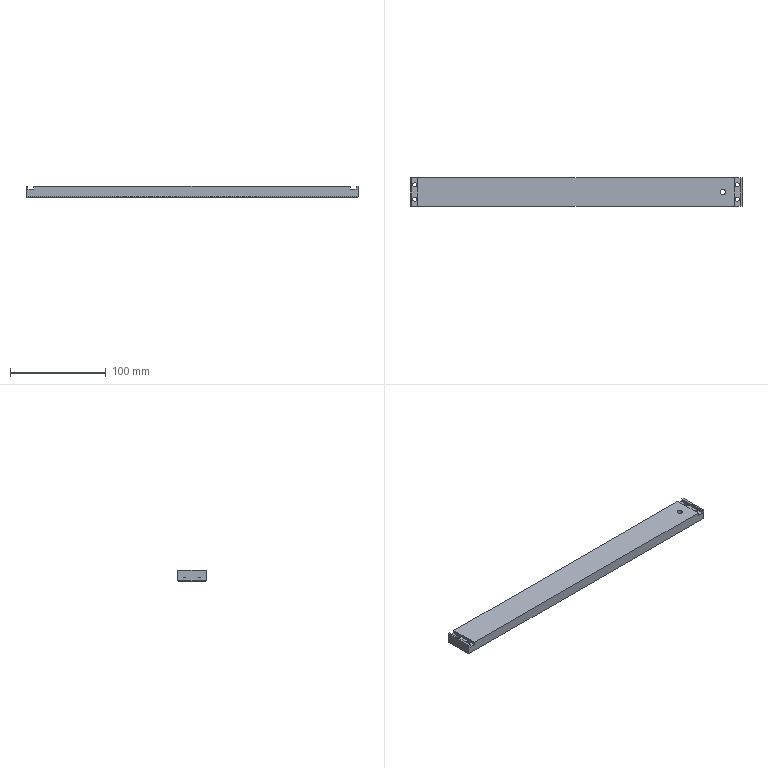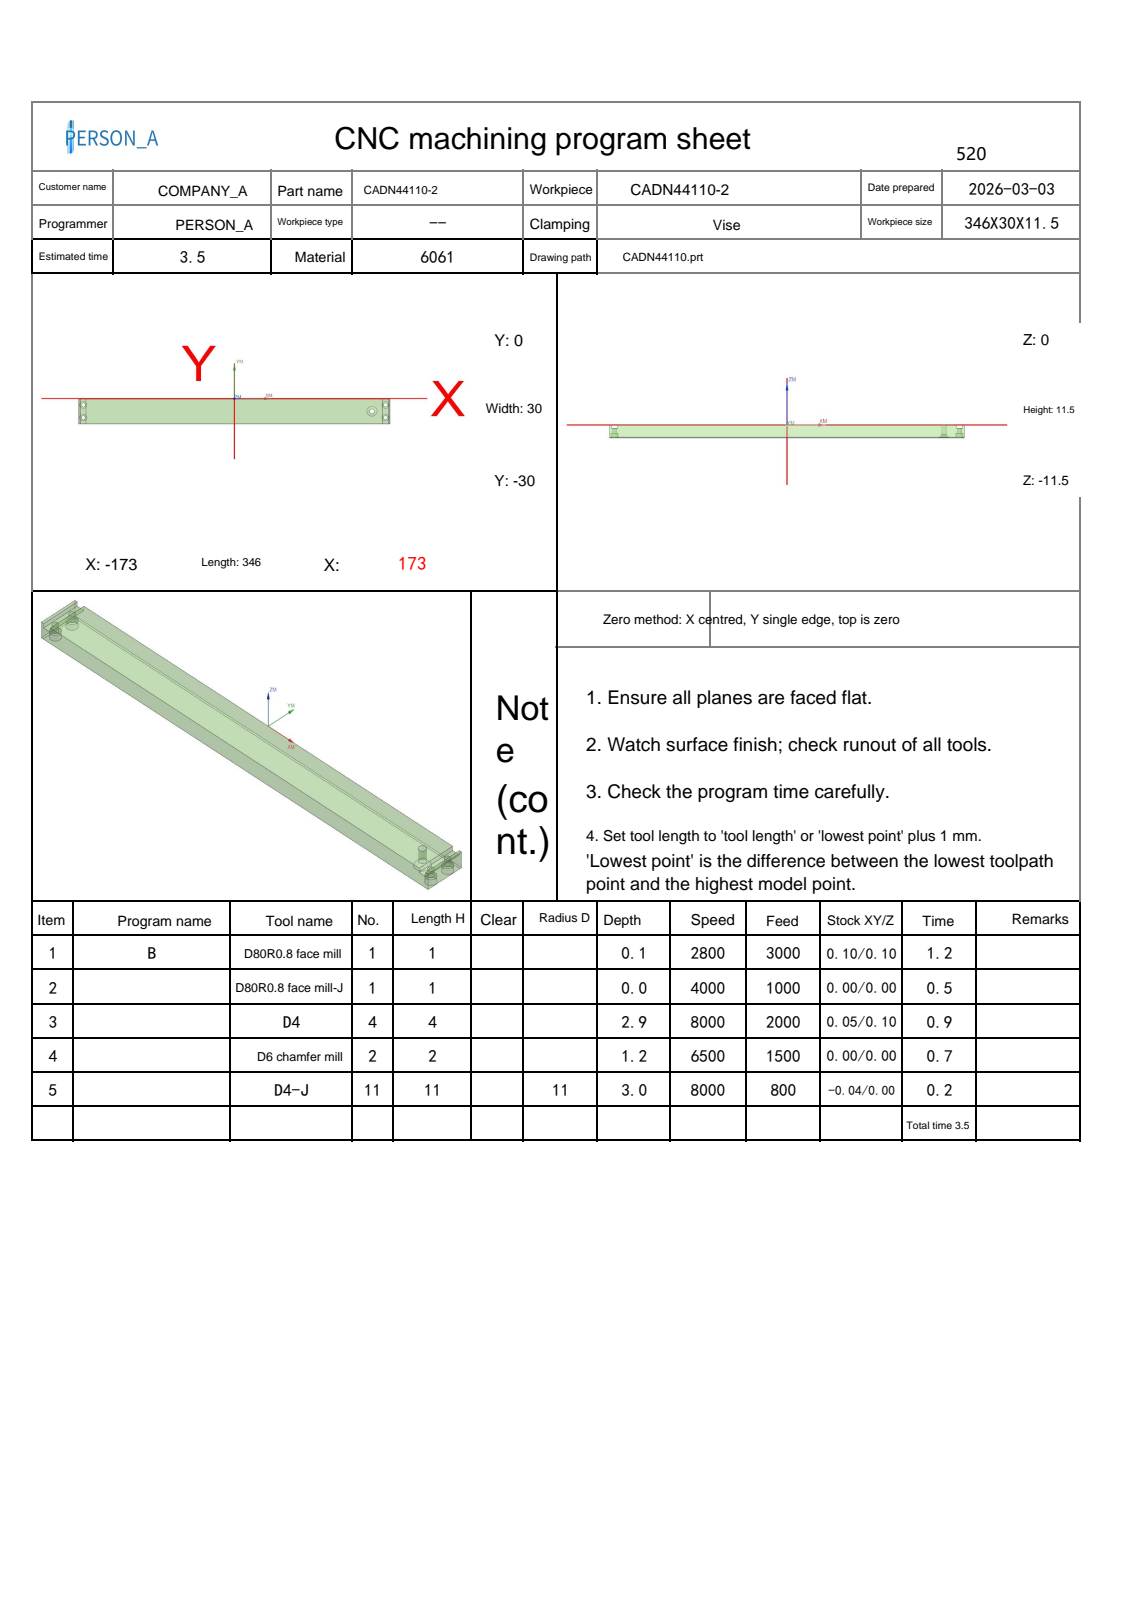NC program | NX | posted by the shop | part box 346 x 30 x 11.5 mm
Whole program:
%
O0001
(Machine time: 4.34 MIN)
(===Total Tool:4===)
(T1=D80R0.8 face mill D=80. R=0.8 D- H01 Z=0.    )
(T4=D4      D=4.   R=0.   D-  H04 Z=-2.9  )
(T2=D6 chamfer mill D=6. R=0. D- H02 Z=-1.2  )
(T11=D4-J   D=4.   R=0.   D11 H11 Z=-3.   )
G80 G90 G17 G49 G40
G91 G28 Z0
M01
N1 T01 M06
(D80R0.8 face mill D=80. R=0.8 H=01 ce=0.10 di=0.10)
G00 G90 G54 X-225.097 Y-15. M03 S2800
G43 H01 Z50.
M08
Z4.517
G01 Z2.517 F3000.
X-213.097
X213.097
X225.097
Z4.517
G00 X-225.097
Z4.033
G01 Z2.033
X-213.097
X213.097
X225.097
Z4.033
G00 X-225.097
Z3.55
G01 Z1.55
X-213.097
X213.097
X225.097
Z3.55
G00 X-225.097
Z3.067
G01 Z1.067
X-213.097
X213.097
X225.097
Z3.067
G00 Z50.
X-225.097
Z2.583
G01 Z.583
X-213.097
X213.097
X225.097
Z2.583
G00 Z50.
X-225.097
Z2.1
G01 Z.1
X-213.097
X213.097
X225.097
Z2.1
G00 Z50.
G91 G28 Z0.0
M05
M09
G91 G28 Z0.0
M01
N2 T01 M06
(D80R0.8 face mill-J D=80. R=0.8 H=01 ce=0.00 di=0.00)
G00 G90 G54 X-224.999 Y-15. M03 S4000
G43 H01 Z50.
M08
Z2.
G01 Z0.0 F1000.
X-212.999
X212.999
X224.999
Z2.
G00 Z50.
G91 G28 Z0.0
M05
M09
G91 G28 Z0.0
M01
N3 T04 M06
(D4  D=4. R=0. H=04 ce=0.05 di=0.10)
G00 G90 G54 X-168. Y-35.05 M03 S8000
G43 H04 Z13.
M08
Z1.21
G01 Z-.29 F2000.
Y-31.96
X-168.95
Y1.96
X-167.05
Y-31.96
X-168.
X-168.5
Y-35.05
Z1.21
G00 X-168.
Z.92
G01 Z-.58
Y-31.96
X-168.95
Y1.96
X-167.05
Y-31.96
X-168.
X-168.5
Y-35.05
Z.92
G00 X-168.
Z.63
G01 Z-.87
Y-31.96
X-168.95
Y1.96
X-167.05
Y-31.96
X-168.
X-168.5
Y-35.05
Z.63
G00 X-168.
Z.34
G01 Z-1.16
Y-31.96
X-168.95
Y1.96
X-167.05
Y-31.96
X-168.
X-168.5
Y-35.05
Z.34
G00 X-168.
Z.05
G01 Z-1.45
Y-31.96
X-168.95
Y1.96
X-167.05
Y-31.96
X-168.
X-168.5
Y-35.05
Z.05
G00 X-168.
Z-.24
G01 Z-1.74
Y-31.96
X-168.95
Y1.96
X-167.05
Y-31.96
X-168.
X-168.5
Y-35.05
Z-.24
G00 X-168.
Z-.53
G01 Z-2.03
Y-31.96
X-168.95
Y1.96
X-167.05
Y-31.96
X-168.
X-168.5
Y-35.05
Z-.53
G00 X-168.
Z-.82
G01 Z-2.32
Y-31.96
X-168.95
Y1.96
X-167.05
Y-31.96
X-168.
X-168.5
Y-35.05
Z-.82
G00 X-168.
Z-1.11
G01 Z-2.61
Y-31.96
X-168.95
Y1.96
X-167.05
Y-31.96
X-168.
X-168.5
Y-35.05
Z-1.11
G00 X-168.
Z-1.4
G01 Z-2.9
Y-31.96
X-168.95
Y1.96
X-167.05
Y-31.96
X-168.
X-168.5
Y-35.05
Z-1.4
G00 Z3.
X168.
Z1.21
G01 Z-.29
Y-31.96
X167.05
Y1.96
X168.95
Y-31.96
X168.
X167.5
Y-35.05
Z1.21
G00 X168.
Z.92
G01 Z-.58
Y-31.96
X167.05
Y1.96
X168.95
Y-31.96
X168.
X167.5
Y-35.05
Z.92
G00 X168.
Z.63
G01 Z-.87
Y-31.96
X167.05
Y1.96
X168.95
Y-31.96
X168.
X167.5
Y-35.05
Z.63
G00 X168.
Z.34
G01 Z-1.16
Y-31.96
X167.05
Y1.96
X168.95
Y-31.96
X168.
X167.5
Y-35.05
Z.34
G00 X168.
Z.05
G01 Z-1.45
Y-31.96
X167.05
Y1.96
X168.95
Y-31.96
X168.
X167.5
Y-35.05
Z.05
G00 X168.
Z-.24
G01 Z-1.74
Y-31.96
X167.05
Y1.96
X168.95
Y-31.96
X168.
X167.5
Y-35.05
Z-.24
G00 X168.
Z-.53
G01 Z-2.03
Y-31.96
X167.05
Y1.96
X168.95
Y-31.96
X168.
X167.5
Y-35.05
Z-.53
G00 X168.
Z-.82
G01 Z-2.32
Y-31.96
X167.05
Y1.96
X168.95
Y-31.96
X168.
X167.5
Y-35.05
Z-.82
G00 X168.
Z-1.11
G01 Z-2.61
Y-31.96
X167.05
Y1.96
X168.95
Y-31.96
X168.
X167.5
Y-35.05
Z-1.11
G00 X168.
Z-1.4
G01 Z-2.9
Y-31.96
X167.05
Y1.96
X168.95
Y-31.96
X168.
X167.5
Y-35.05
Z-1.4
G00 Z13.
G91 G28 Z0.0
M05
M09
G91 G28 Z0.0
M01
N4 T02 M06
(D6 chamfer mill D=6. R=0. H=02 ce=0.00 di=0.00)
G00 G90 G54 X.386 Y-31.227 M03 S6500
G43 H02 Z50.
M08
Z.172
G01 Z-1.2 F1500.
G03 X.1 Y-31.027 I-1.286 J-1.532
G01 X.054 Y-30.997
X0.0 Y-31.
X-165.
G02 X-166. Y-30. I0.0 J1.
G01 Y0.0
G02 X-165. Y1. I1. J0.0
G01 X165.
G02 X166. Y0.0 I0.0 J-1.
G01 Y-30.
G02 X165. Y-31. I-1. J0.0
G01 X0.0
X-.054 Y-30.997
X-.1 Y-31.027
G03 X-.386 Y-31.227 I1. J-1.732
G01 Z.172
G00 Z10.
X154.565 Y-15.407
Z.27
G01 Z-1.2
G03 X154.734 Y-15.102 I-1.658 J1.118
G01 X154.759 Y-15.054
X154.75 Y-15.
G03 X153. Y-13.25 I-1.75 J0.0
X151.25 Y-15. I0.0 J-1.75
X153. Y-16.75 I1.75 J0.0
X154.75 Y-15. I0.0 J1.75
G01 X154.759 Y-14.946
X154.734 Y-14.898
G03 X154.565 Y-14.593 I-1.827 J-.813
G01 Z.27
G00 Z10.
X-169.773 Y-14.614
Z.172
G01 Z-1.2
G03 X-169.973 Y-14.9 I1.532 J-1.286
G01 X-170.003 Y-14.946
X-170. Y-15.
Y-30.
G02 X-171. Y-31. I-1. J0.0
G01 X-173.
G02 X-174. Y-30. I0.0 J1.
G01 Y0.0
G02 X-173. Y1. I1. J0.0
G01 X-171.
G02 X-170. Y0.0 I0.0 J-1.
G01 Y-15.
X-170.003 Y-15.054
X-169.973 Y-15.1
G03 X-169.773 Y-15.386 I1.732 J1.
G01 Z.172
G00 Z10.
X169.773
Z.172
G01 Z-1.2
G03 X169.973 Y-15.1 I-1.532 J1.286
G01 X170.003 Y-15.054
X170. Y-15.
Y0.0
G02 X171. Y1. I1. J0.0
G01 X173.
G02 X174. Y0.0 I0.0 J-1.
G01 Y-30.
G02 X173. Y-31. I-1. J0.0
G01 X171.
G02 X170. Y-30. I0.0 J1.
G01 Y-15.
X170.003 Y-14.946
X169.973 Y-14.9
G03 X169.773 Y-14.614 I-1.732 J-1.
G01 Z.172
G00 Z50.
G91 G28 Z0.0
M05
M09
G91 G28 Z0.0
M01
N5 T11 M06
(D4-J  D=4. R=0. H=11 ce=-0.04 di=0.00)
G00 G90 G54 X168.321 Y-32.821 M03 S8000
G43 H11 Z13.
M08
Z-2.
G01 Z-3. F800.
G41 D11
X168.51 Y-32.755
G03 X169.045 Y-32. I-.265 J.755
G01 Y2.
G03 X168.51 Y2.755 I-.8 J0.0
G01 G40 X168.321 Y2.821
X167.679
G41 D11
X167.49 Y2.755
G03 X166.955 Y2. I.265 J-.755
G01 Y-32.
G03 X167.49 Y-32.755 I.8 J0.0
G01 G40 X167.679 Y-32.821
Z-2.
G00 Z3.
X-167.679
Z-2.
G01 Z-3.
G41 D11
X-167.49 Y-32.755
G03 X-166.955 Y-32. I-.265 J.755
G01 Y2.
G03 X-167.49 Y2.755 I-.8 J0.0
G01 G40 X-167.679 Y2.821
X-168.321
G41 D11
X-168.51 Y2.755
G03 X-169.045 Y2. I.265 J-.755
G01 Y-32.
G03 X-168.51 Y-32.755 I.8 J0.0
G01 G40 X-168.321 Y-32.821
Z-2.
G00 Z13.
M05
M09
G91 G28 Z0.0
G91 G28 Y0.0
M30
%